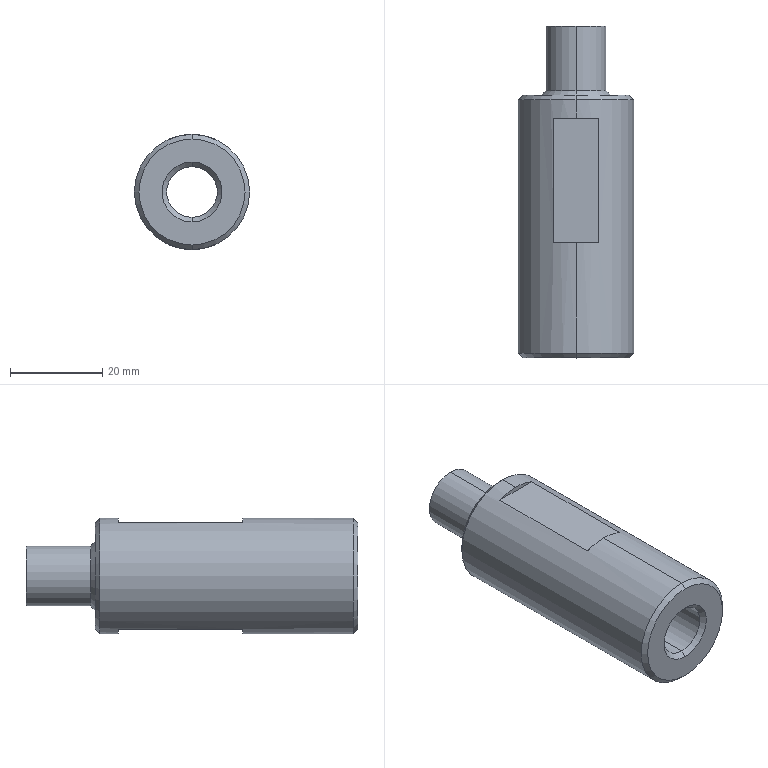Part | STEP file | 1 solid | 24 faces | box 25 x 72 x 25 mm | volume 22681 mm3 | cone 10 | plane 8 | cylinder 6 | commonest cylinder face diameters 11 x2 13 x2 25 x2